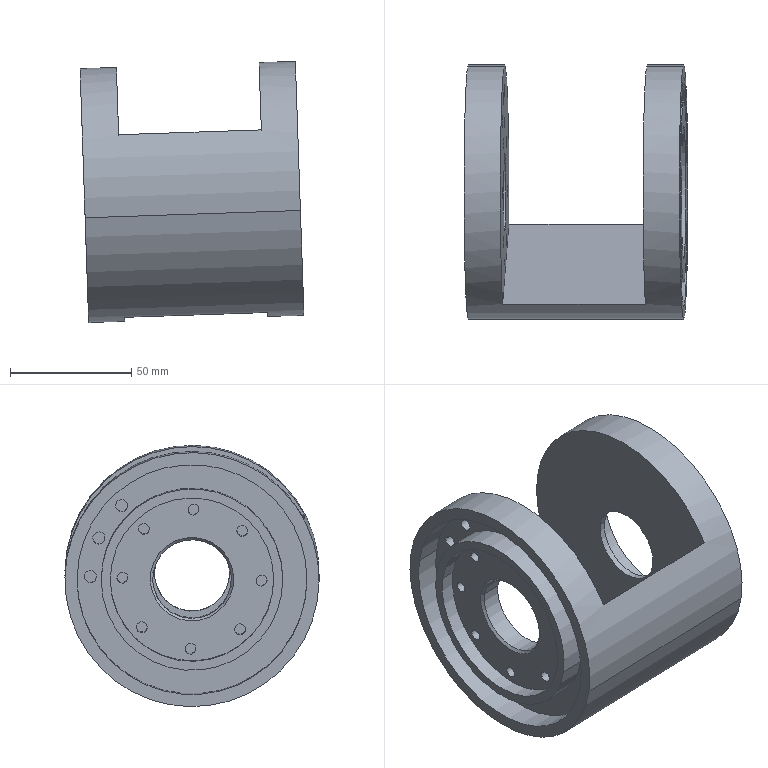Part | STEP file | 2026.6.15-Main Assembly图.sldasm-Part-135 | 1 solid | 56 faces | box 92.5 x 105 x 107.949 mm | volume 212796 mm3 | cylinder 42 | plane 12 | cone 2 | commonest cylinder face diameters 4.5 x16 5 x6 75 x4 95 x4 31 x2 32.5 x2